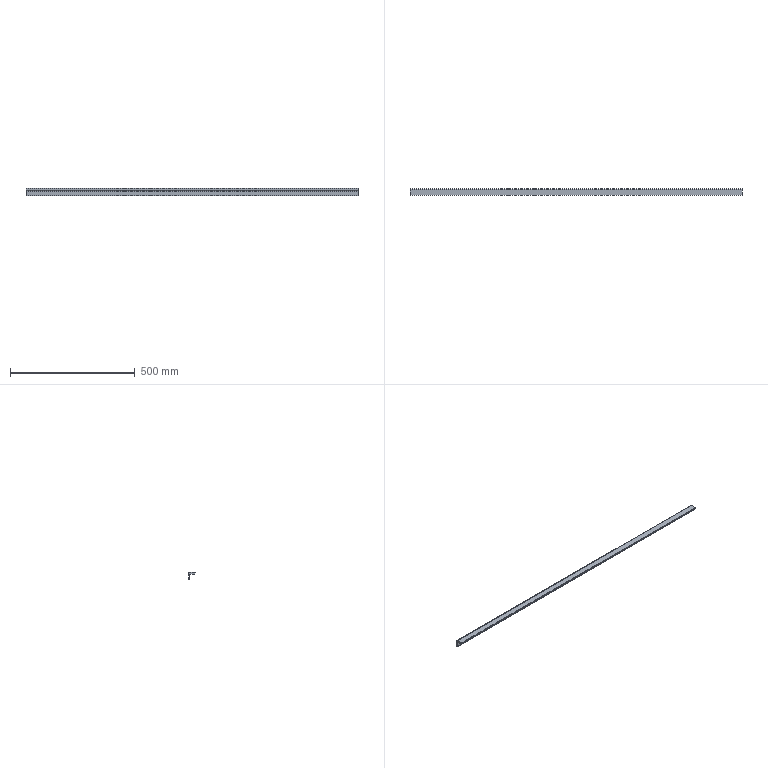Part | SolidWorks | features BaseBody 1 | 1 solid | 24 faces | box 1330 x 28 x 29.5 mm | volume 384644 mm3 | plane 19 | cylinder 5 | commonest cylinder face diameters 0.6 x3 8 x1 10 x1
STEP:
#1=CARTESIAN_POINT('',(-671.521,190.,396.5));
#2=VERTEX_POINT('',#1);
#3=CARTESIAN_POINT('',(-671.521,190.3,396.2));
#4=VERTEX_POINT('',#3);
#5=CARTESIAN_POINT('',(-671.521,190.3,396.5));
#6=DIRECTION('',(1.,0.,0.));
#7=DIRECTION('',(0.,0.,-1.));
#8=AXIS2_PLACEMENT_3D('',#5,#6,#7);
#9=CIRCLE('',#8,0.3);
#10=EDGE_CURVE('',#2,#4,#9,.T.);
#11=ORIENTED_EDGE('',*,*,#10,.T.);
#12=CARTESIAN_POINT('',(658.479,190.3,396.2));
#13=VERTEX_POINT('',#12);
#14=CARTESIAN_POINT('',(68.479,190.3,396.2));
#15=DIRECTION('',(1.,0.,0.));
#16=VECTOR('',#15,1000.);
#17=LINE('',#14,#16);
#18=EDGE_CURVE('',#4,#13,#17,.T.);
#19=ORIENTED_EDGE('',*,*,#18,.T.);
#20=CARTESIAN_POINT('',(658.479,190.,396.5));
#21=VERTEX_POINT('',#20);
#22=CARTESIAN_POINT('',(658.479,190.3,396.5));
#23=DIRECTION('',(1.,0.,0.));
#24=DIRECTION('',(0.,0.,-1.));
#25=AXIS2_PLACEMENT_3D('',#22,#23,#24);
#26=CIRCLE('',#25,0.3);
#27=EDGE_CURVE('',#21,#13,#26,.T.);
#28=ORIENTED_EDGE('',*,*,#27,.F.);
#29=CARTESIAN_POINT('',(68.479,190.,396.5));
#30=DIRECTION('',(-1.,0.,0.));
#31=VECTOR('',#30,1000.);
#32=LINE('',#29,#31);
#33=EDGE_CURVE('',#21,#2,#32,.T.);
#34=ORIENTED_EDGE('',*,*,#33,.T.);
#35=EDGE_LOOP('',(#11,#19,#28,#34));
#36=FACE_OUTER_BOUND('',#35,.T.);
#37=CARTESIAN_POINT('',(68.479,190.3,396.5));
#38=DIRECTION('',(1.,0.,0.));
#39=DIRECTION('',(0.,0.,-1.));
#40=AXIS2_PLACEMENT_3D('',#37,#38,#39);
#41=CYLINDRICAL_SURFACE('',#40,0.3);
#42=ADVANCED_FACE('',(#36),#41,.T.);
#43=CARTESIAN_POINT('',(658.479,187.,420.));
#44=VERTEX_POINT('',#43);
#45=CARTESIAN_POINT('',(-671.521,187.,420.));
#46=VERTEX_POINT('',#45);
#47=CARTESIAN_POINT('',(68.479,187.,420.));
#48=DIRECTION('',(-1.,0.,0.));
#49=VECTOR('',#48,1000.);
#50=LINE('',#47,#49);
#51=EDGE_CURVE('',#44,#46,#50,.T.);
#52=ORIENTED_EDGE('',*,*,#51,.T.);
#53=CARTESIAN_POINT('',(-671.521,164.,420.));
#54=VERTEX_POINT('',#53);
#55=CARTESIAN_POINT('',(-671.521,164.,420.));
#56=DIRECTION('',(0.,-1.,0.));
#57=VECTOR('',#56,1000.);
#58=LINE('',#55,#57);
#59=EDGE_CURVE('',#46,#54,#58,.T.);
#60=ORIENTED_EDGE('',*,*,#59,.T.);
#61=CARTESIAN_POINT('',(658.479,164.,420.));
#62=VERTEX_POINT('',#61);
#63=CARTESIAN_POINT('',(68.479,164.,420.));
#64=DIRECTION('',(1.,0.,0.));
#65=VECTOR('',#64,1000.);
#66=LINE('',#63,#65);
#67=EDGE_CURVE('',#54,#62,#66,.T.);
#68=ORIENTED_EDGE('',*,*,#67,.T.);
#69=CARTESIAN_POINT('',(658.479,164.,420.));
#70=DIRECTION('',(0.,1.,0.));
#71=VECTOR('',#70,1000.);
#72=LINE('',#69,#71);
#73=EDGE_CURVE('',#62,#44,#72,.T.);
#74=ORIENTED_EDGE('',*,*,#73,.T.);
#75=EDGE_LOOP('',(#52,#60,#68,#74));
#76=FACE_OUTER_BOUND('',#75,.T.);
#77=CARTESIAN_POINT('',(68.479,164.,420.));
#78=DIRECTION('',(0.,0.,1.));
#79=DIRECTION('',(0.,-1.,0.));
#80=AXIS2_PLACEMENT_3D('',#77,#78,#79);
#81=PLANE('',#80);
#82=ADVANCED_FACE('',(#76),#81,.T.);
#83=CARTESIAN_POINT('',(-671.521,164.,418.));
#84=VERTEX_POINT('',#83);
#85=CARTESIAN_POINT('',(-671.521,164.,408.659));
#86=DIRECTION('',(0.,0.,-1.));
#87=VECTOR('',#86,1000.);
#88=LINE('',#85,#87);
#89=EDGE_CURVE('',#54,#84,#88,.T.);
#90=ORIENTED_EDGE('',*,*,#89,.F.);
#91=ORIENTED_EDGE('',*,*,#59,.F.);
#92=CARTESIAN_POINT('',(-671.521,192.,415.));
#93=VERTEX_POINT('',#92);
#94=CARTESIAN_POINT('',(-671.521,187.,415.));
#95=DIRECTION('',(1.,0.,0.));
#96=DIRECTION('',(0.,0.,-1.));
#97=AXIS2_PLACEMENT_3D('',#94,#95,#96);
#98=CIRCLE('',#97,5.);
#99=EDGE_CURVE('',#93,#46,#98,.T.);
#100=ORIENTED_EDGE('',*,*,#99,.F.);
#101=CARTESIAN_POINT('',(-671.521,192.,400.7));
#102=VERTEX_POINT('',#101);
#103=CARTESIAN_POINT('',(-671.521,192.,408.659));
#104=DIRECTION('',(0.,0.,1.));
#105=VECTOR('',#104,1000.);
#106=LINE('',#103,#105);
#107=EDGE_CURVE('',#102,#93,#106,.T.);
#108=ORIENTED_EDGE('',*,*,#107,.F.);
#109=CARTESIAN_POINT('',(-671.521,191.8,400.5));
#110=VERTEX_POINT('',#109);
#111=CARTESIAN_POINT('',(-671.521,191.8,400.5));
#112=DIRECTION('',(0.,0.7071,0.7071));
#113=VECTOR('',#112,1000.);
#114=LINE('',#111,#113);
#115=EDGE_CURVE('',#110,#102,#114,.T.);
#116=ORIENTED_EDGE('',*,*,#115,.F.);
#117=CARTESIAN_POINT('',(-671.521,191.8,396.5));
#118=VERTEX_POINT('',#117);
#119=CARTESIAN_POINT('',(-671.521,191.8,408.659));
#120=DIRECTION('',(0.,0.,1.));
#121=VECTOR('',#120,1000.);
#122=LINE('',#119,#121);
#123=EDGE_CURVE('',#118,#110,#122,.T.);
#124=ORIENTED_EDGE('',*,*,#123,.F.);
#125=CARTESIAN_POINT('',(-671.521,190.6,396.5));
#126=VERTEX_POINT('',#125);
#127=CARTESIAN_POINT('',(-671.521,182.62,396.5));
#128=DIRECTION('',(0.,1.,0.));
#129=VECTOR('',#128,1000.);
#130=LINE('',#127,#129);
#131=EDGE_CURVE('',#126,#118,#130,.T.);
#132=ORIENTED_EDGE('',*,*,#131,.F.);
#133=CARTESIAN_POINT('',(-671.521,190.3,396.5));
#134=DIRECTION('',(1.,0.,0.));
#135=DIRECTION('',(0.,0.,-1.));
#136=AXIS2_PLACEMENT_3D('',#133,#134,#135);
#137=CIRCLE('',#136,0.3);
#138=EDGE_CURVE('',#4,#126,#137,.T.);
#139=ORIENTED_EDGE('',*,*,#138,.F.);
#140=ORIENTED_EDGE('',*,*,#10,.F.);
#141=CARTESIAN_POINT('',(-671.521,188.8,396.5));
#142=VERTEX_POINT('',#141);
#143=CARTESIAN_POINT('',(-671.521,182.62,396.5));
#144=DIRECTION('',(0.,1.,0.));
#145=VECTOR('',#144,1000.);
#146=LINE('',#143,#145);
#147=EDGE_CURVE('',#142,#2,#146,.T.);
#148=ORIENTED_EDGE('',*,*,#147,.F.);
#149=CARTESIAN_POINT('',(-671.521,188.8,392.5));
#150=VERTEX_POINT('',#149);
#151=CARTESIAN_POINT('',(-671.521,188.8,408.659));
#152=DIRECTION('',(0.,0.,1.));
#153=VECTOR('',#152,1000.);
#154=LINE('',#151,#153);
#155=EDGE_CURVE('',#150,#142,#154,.T.);
#156=ORIENTED_EDGE('',*,*,#155,.F.);
#157=CARTESIAN_POINT('',(-671.521,190.,392.5));
#158=VERTEX_POINT('',#157);
#159=CARTESIAN_POINT('',(-671.521,182.62,392.5));
#160=DIRECTION('',(0.,-1.,0.));
#161=VECTOR('',#160,1000.);
#162=LINE('',#159,#161);
#163=EDGE_CURVE('',#158,#150,#162,.T.);
#164=ORIENTED_EDGE('',*,*,#163,.F.);
#165=CARTESIAN_POINT('',(-671.521,190.6,392.5));
#166=VERTEX_POINT('',#165);
#167=CARTESIAN_POINT('',(-671.521,190.3,392.5));
#168=DIRECTION('',(1.,0.,0.));
#169=DIRECTION('',(0.,0.,-1.));
#170=AXIS2_PLACEMENT_3D('',#167,#168,#169);
#171=CIRCLE('',#170,0.3);
#172=EDGE_CURVE('',#166,#158,#171,.T.);
#173=ORIENTED_EDGE('',*,*,#172,.F.);
#174=CARTESIAN_POINT('',(-671.521,191.8,392.5));
#175=VERTEX_POINT('',#174);
#176=CARTESIAN_POINT('',(-671.521,182.62,392.5));
#177=DIRECTION('',(0.,-1.,0.));
#178=VECTOR('',#177,1000.);
#179=LINE('',#176,#178);
#180=EDGE_CURVE('',#175,#166,#179,.T.);
#181=ORIENTED_EDGE('',*,*,#180,.F.);
#182=CARTESIAN_POINT('',(-671.521,191.8,390.5));
#183=VERTEX_POINT('',#182);
#184=CARTESIAN_POINT('',(-671.521,191.8,408.659));
#185=DIRECTION('',(0.,0.,1.));
#186=VECTOR('',#185,1000.);
#187=LINE('',#184,#186);
#188=EDGE_CURVE('',#183,#175,#187,.T.);
#189=ORIENTED_EDGE('',*,*,#188,.F.);
#190=CARTESIAN_POINT('',(-671.521,187.,390.5));
#191=VERTEX_POINT('',#190);
#192=CARTESIAN_POINT('',(-671.521,182.62,390.5));
#193=DIRECTION('',(0.,1.,0.));
#194=VECTOR('',#193,1000.);
#195=LINE('',#192,#194);
#196=EDGE_CURVE('',#191,#183,#195,.T.);
#197=ORIENTED_EDGE('',*,*,#196,.F.);
#198=CARTESIAN_POINT('',(-671.521,187.,408.5));
#199=VERTEX_POINT('',#198);
#200=CARTESIAN_POINT('',(-671.521,187.,408.659));
#201=DIRECTION('',(0.,0.,-1.));
#202=VECTOR('',#201,1000.);
#203=LINE('',#200,#202);
#204=EDGE_CURVE('',#199,#191,#203,.T.);
#205=ORIENTED_EDGE('',*,*,#204,.F.);
#206=CARTESIAN_POINT('',(-671.521,183.,412.5));
#207=VERTEX_POINT('',#206);
#208=CARTESIAN_POINT('',(-671.521,183.,408.5));
#209=DIRECTION('',(-1.,0.,0.));
#210=DIRECTION('',(0.,0.,-1.));
#211=AXIS2_PLACEMENT_3D('',#208,#209,#210);
#212=CIRCLE('',#211,4.);
#213=EDGE_CURVE('',#207,#199,#212,.T.);
#214=ORIENTED_EDGE('',*,*,#213,.F.);
#215=CARTESIAN_POINT('',(-671.521,167.,412.5));
#216=VERTEX_POINT('',#215);
#217=CARTESIAN_POINT('',(-671.521,182.62,412.5));
#218=DIRECTION('',(0.,1.,0.));
#219=VECTOR('',#218,1000.);
#220=LINE('',#217,#219);
#221=EDGE_CURVE('',#216,#207,#220,.T.);
#222=ORIENTED_EDGE('',*,*,#221,.F.);
#223=CARTESIAN_POINT('',(-671.521,167.,417.5));
#224=VERTEX_POINT('',#223);
#225=CARTESIAN_POINT('',(-671.521,167.,408.659));
#226=DIRECTION('',(0.,0.,-1.));
#227=VECTOR('',#226,1000.);
#228=LINE('',#225,#227);
#229=EDGE_CURVE('',#224,#216,#228,.T.);
#230=ORIENTED_EDGE('',*,*,#229,.F.);
#231=CARTESIAN_POINT('',(-671.521,164.5,417.5));
#232=VERTEX_POINT('',#231);
#233=CARTESIAN_POINT('',(-671.521,182.62,417.5));
#234=DIRECTION('',(0.,1.,0.));
#235=VECTOR('',#234,1000.);
#236=LINE('',#233,#235);
#237=EDGE_CURVE('',#232,#224,#236,.T.);
#238=ORIENTED_EDGE('',*,*,#237,.F.);
#239=CARTESIAN_POINT('',(-671.521,164.,418.));
#240=DIRECTION('',(0.,0.7071,-0.7071));
#241=VECTOR('',#240,1000.);
#242=LINE('',#239,#241);
#243=EDGE_CURVE('',#84,#232,#242,.T.);
#244=ORIENTED_EDGE('',*,*,#243,.F.);
#245=EDGE_LOOP('',(#90,#91,#100,#108,#116,#124,#132,#139,#140,#148,#156,#164,#173,#181,#189,#197,#205,#214,#222,#230,#238,#244));
#246=FACE_OUTER_BOUND('',#245,.T.);
#247=CARTESIAN_POINT('',(-671.521,182.62,408.659));
#248=DIRECTION('',(1.,0.,0.));
#249=DIRECTION('',(0.,0.,-1.));
#250=AXIS2_PLACEMENT_3D('',#247,#248,#249);
#251=PLANE('',#250);
#252=ADVANCED_FACE('',(#246),#251,.F.);
#253=CARTESIAN_POINT('',(658.479,192.,415.));
#254=VERTEX_POINT('',#253);
#255=CARTESIAN_POINT('',(68.479,192.,415.));
#256=DIRECTION('',(-1.,0.,0.));
#257=VECTOR('',#256,1000.);
#258=LINE('',#255,#257);
#259=EDGE_CURVE('',#254,#93,#258,.T.);
#260=ORIENTED_EDGE('',*,*,#259,.T.);
#261=ORIENTED_EDGE('',*,*,#99,.T.);
#262=ORIENTED_EDGE('',*,*,#51,.F.);
#263=CARTESIAN_POINT('',(658.479,187.,415.));
#264=DIRECTION('',(-1.,0.,0.));
#265=DIRECTION('',(0.,0.,-1.));
#266=AXIS2_PLACEMENT_3D('',#263,#264,#265);
#267=CIRCLE('',#266,5.);
#268=EDGE_CURVE('',#44,#254,#267,.T.);
#269=ORIENTED_EDGE('',*,*,#268,.T.);
#270=EDGE_LOOP('',(#260,#261,#262,#269));
#271=FACE_OUTER_BOUND('',#270,.T.);
#272=CARTESIAN_POINT('',(68.479,187.,415.));
#273=DIRECTION('',(1.,0.,0.));
#274=DIRECTION('',(0.,0.,-1.));
#275=AXIS2_PLACEMENT_3D('',#272,#273,#274);
#276=CYLINDRICAL_SURFACE('',#275,5.);
#277=ADVANCED_FACE('',(#271),#276,.T.);
#278=ORIENTED_EDGE('',*,*,#73,.F.);
#279=CARTESIAN_POINT('',(658.479,164.,418.));
#280=VERTEX_POINT('',#279);
#281=CARTESIAN_POINT('',(658.479,164.,408.659));
#282=DIRECTION('',(0.,0.,-1.));
#283=VECTOR('',#282,1000.);
#284=LINE('',#281,#283);
#285=EDGE_CURVE('',#62,#280,#284,.T.);
#286=ORIENTED_EDGE('',*,*,#285,.T.);
#287=CARTESIAN_POINT('',(658.479,164.5,417.5));
#288=VERTEX_POINT('',#287);
#289=CARTESIAN_POINT('',(658.479,164.,418.));
#290=DIRECTION('',(0.,0.7071,-0.7071));
#291=VECTOR('',#290,1000.);
#292=LINE('',#289,#291);
#293=EDGE_CURVE('',#280,#288,#292,.T.);
#294=ORIENTED_EDGE('',*,*,#293,.T.);
#295=CARTESIAN_POINT('',(658.479,167.,417.5));
#296=VERTEX_POINT('',#295);
#297=CARTESIAN_POINT('',(658.479,182.62,417.5));
#298=DIRECTION('',(0.,1.,0.));
#299=VECTOR('',#298,1000.);
#300=LINE('',#297,#299);
#301=EDGE_CURVE('',#288,#296,#300,.T.);
#302=ORIENTED_EDGE('',*,*,#301,.T.);
#303=CARTESIAN_POINT('',(658.479,167.,412.5));
#304=VERTEX_POINT('',#303);
#305=CARTESIAN_POINT('',(658.479,167.,408.659));
#306=DIRECTION('',(0.,0.,-1.));
#307=VECTOR('',#306,1000.);
#308=LINE('',#305,#307);
#309=EDGE_CURVE('',#296,#304,#308,.T.);
#310=ORIENTED_EDGE('',*,*,#309,.T.);
#311=CARTESIAN_POINT('',(658.479,183.,412.5));
#312=VERTEX_POINT('',#311);
#313=CARTESIAN_POINT('',(658.479,182.62,412.5));
#314=DIRECTION('',(0.,1.,0.));
#315=VECTOR('',#314,1000.);
#316=LINE('',#313,#315);
#317=EDGE_CURVE('',#304,#312,#316,.T.);
#318=ORIENTED_EDGE('',*,*,#317,.T.);
#319=CARTESIAN_POINT('',(658.479,187.,408.5));
#320=VERTEX_POINT('',#319);
#321=CARTESIAN_POINT('',(658.479,183.,408.5));
#322=DIRECTION('',(-1.,0.,0.));
#323=DIRECTION('',(0.,0.,-1.));
#324=AXIS2_PLACEMENT_3D('',#321,#322,#323);
#325=CIRCLE('',#324,4.);
#326=EDGE_CURVE('',#312,#320,#325,.T.);
#327=ORIENTED_EDGE('',*,*,#326,.T.);
#328=CARTESIAN_POINT('',(658.479,187.,390.5));
#329=VERTEX_POINT('',#328);
#330=CARTESIAN_POINT('',(658.479,187.,408.659));
#331=DIRECTION('',(0.,0.,-1.));
#332=VECTOR('',#331,1000.);
#333=LINE('',#330,#332);
#334=EDGE_CURVE('',#320,#329,#333,.T.);
#335=ORIENTED_EDGE('',*,*,#334,.T.);
#336=CARTESIAN_POINT('',(658.479,191.8,390.5));
#337=VERTEX_POINT('',#336);
#338=CARTESIAN_POINT('',(658.479,182.62,390.5));
#339=DIRECTION('',(0.,1.,0.));
#340=VECTOR('',#339,1000.);
#341=LINE('',#338,#340);
#342=EDGE_CURVE('',#329,#337,#341,.T.);
#343=ORIENTED_EDGE('',*,*,#342,.T.);
#344=CARTESIAN_POINT('',(658.479,191.8,392.5));
#345=VERTEX_POINT('',#344);
#346=CARTESIAN_POINT('',(658.479,191.8,408.659));
#347=DIRECTION('',(0.,0.,1.));
#348=VECTOR('',#347,1000.);
#349=LINE('',#346,#348);
#350=EDGE_CURVE('',#337,#345,#349,.T.);
#351=ORIENTED_EDGE('',*,*,#350,.T.);
#352=CARTESIAN_POINT('',(658.479,190.6,392.5));
#353=VERTEX_POINT('',#352);
#354=CARTESIAN_POINT('',(658.479,182.62,392.5));
#355=DIRECTION('',(0.,-1.,0.));
#356=VECTOR('',#355,1000.);
#357=LINE('',#354,#356);
#358=EDGE_CURVE('',#345,#353,#357,.T.);
#359=ORIENTED_EDGE('',*,*,#358,.T.);
#360=CARTESIAN_POINT('',(658.479,190.,392.5));
#361=VERTEX_POINT('',#360);
#362=CARTESIAN_POINT('',(658.479,190.3,392.5));
#363=DIRECTION('',(1.,0.,0.));
#364=DIRECTION('',(0.,0.,-1.));
#365=AXIS2_PLACEMENT_3D('',#362,#363,#364);
#366=CIRCLE('',#365,0.3);
#367=EDGE_CURVE('',#353,#361,#366,.T.);
#368=ORIENTED_EDGE('',*,*,#367,.T.);
#369=CARTESIAN_POINT('',(658.479,188.8,392.5));
#370=VERTEX_POINT('',#369);
#371=CARTESIAN_POINT('',(658.479,182.62,392.5));
#372=DIRECTION('',(0.,-1.,0.));
#373=VECTOR('',#372,1000.);
#374=LINE('',#371,#373);
#375=EDGE_CURVE('',#361,#370,#374,.T.);
#376=ORIENTED_EDGE('',*,*,#375,.T.);
#377=CARTESIAN_POINT('',(658.479,188.8,396.5));
#378=VERTEX_POINT('',#377);
#379=CARTESIAN_POINT('',(658.479,188.8,408.659));
#380=DIRECTION('',(0.,0.,1.));
#381=VECTOR('',#380,1000.);
#382=LINE('',#379,#381);
#383=EDGE_CURVE('',#370,#378,#382,.T.);
#384=ORIENTED_EDGE('',*,*,#383,.T.);
#385=CARTESIAN_POINT('',(658.479,182.62,396.5));
#386=DIRECTION('',(0.,1.,0.));
#387=VECTOR('',#386,1000.);
#388=LINE('',#385,#387);
#389=EDGE_CURVE('',#378,#21,#388,.T.);
#390=ORIENTED_EDGE('',*,*,#389,.T.);
#391=ORIENTED_EDGE('',*,*,#27,.T.);
#392=CARTESIAN_POINT('',(658.479,190.6,396.5));
#393=VERTEX_POINT('',#392);
#394=CARTESIAN_POINT('',(658.479,190.3,396.5));
#395=DIRECTION('',(1.,0.,0.));
#396=DIRECTION('',(0.,0.,-1.));
#397=AXIS2_PLACEMENT_3D('',#394,#395,#396);
#398=CIRCLE('',#397,0.3);
#399=EDGE_CURVE('',#13,#393,#398,.T.);
#400=ORIENTED_EDGE('',*,*,#399,.T.);
#401=CARTESIAN_POINT('',(658.479,191.8,396.5));
#402=VERTEX_POINT('',#401);
#403=CARTESIAN_POINT('',(658.479,182.62,396.5));
#404=DIRECTION('',(0.,1.,0.));
#405=VECTOR('',#404,1000.);
#406=LINE('',#403,#405);
#407=EDGE_CURVE('',#393,#402,#406,.T.);
#408=ORIENTED_EDGE('',*,*,#407,.T.);
#409=CARTESIAN_POINT('',(658.479,191.8,400.5));
#410=VERTEX_POINT('',#409);
#411=CARTESIAN_POINT('',(658.479,191.8,408.659));
#412=DIRECTION('',(0.,0.,1.));
#413=VECTOR('',#412,1000.);
#414=LINE('',#411,#413);
#415=EDGE_CURVE('',#402,#410,#414,.T.);
#416=ORIENTED_EDGE('',*,*,#415,.T.);
#417=CARTESIAN_POINT('',(658.479,192.,400.7));
#418=VERTEX_POINT('',#417);
#419=CARTESIAN_POINT('',(658.479,191.8,400.5));
#420=DIRECTION('',(0.,0.7071,0.7071));
#421=VECTOR('',#420,1000.);
#422=LINE('',#419,#421);
#423=EDGE_CURVE('',#410,#418,#422,.T.);
#424=ORIENTED_EDGE('',*,*,#423,.T.);
#425=CARTESIAN_POINT('',(658.479,192.,408.659));
#426=DIRECTION('',(0.,0.,1.));
#427=VECTOR('',#426,1000.);
#428=LINE('',#425,#427);
#429=EDGE_CURVE('',#418,#254,#428,.T.);
#430=ORIENTED_EDGE('',*,*,#429,.T.);
#431=ORIENTED_EDGE('',*,*,#268,.F.);
#432=EDGE_LOOP('',(#278,#286,#294,#302,#310,#318,#327,#335,#343,#351,#359,#368,#376,#384,#390,#391,#400,#408,#416,#424,#430,#431));
#433=FACE_OUTER_BOUND('',#432,.T.);
#434=CARTESIAN_POINT('',(658.479,182.62,408.659));
#435=DIRECTION('',(1.,0.,0.));
#436=DIRECTION('',(0.,0.,-1.));
#437=AXIS2_PLACEMENT_3D('',#434,#435,#436);
#438=PLANE('',#437);
#439=ADVANCED_FACE('',(#433),#438,.T.);
#440=ORIENTED_EDGE('',*,*,#67,.F.);
#441=ORIENTED_EDGE('',*,*,#89,.T.);
#442=CARTESIAN_POINT('',(68.479,164.,418.));
#443=DIRECTION('',(1.,0.,0.));
#444=VECTOR('',#443,1000.);
#445=LINE('',#442,#444);
#446=EDGE_CURVE('',#84,#280,#445,.T.);
#447=ORIENTED_EDGE('',*,*,#446,.T.);
#448=ORIENTED_EDGE('',*,*,#285,.F.);
#449=EDGE_LOOP('',(#440,#441,#447,#448));
#450=FACE_OUTER_BOUND('',#449,.T.);
#451=CARTESIAN_POINT('',(68.479,164.,418.));
#452=DIRECTION('',(0.,-1.,0.));
#453=DIRECTION('',(0.,0.,-1.));
#454=AXIS2_PLACEMENT_3D('',#451,#452,#453);
#455=PLANE('',#454);
#456=ADVANCED_FACE('',(#450),#455,.T.);
#457=ORIENTED_EDGE('',*,*,#446,.F.);
#458=ORIENTED_EDGE('',*,*,#243,.T.);
#459=CARTESIAN_POINT('',(68.479,164.5,417.5));
#460=DIRECTION('',(1.,0.,0.));
#461=VECTOR('',#460,1000.);
#462=LINE('',#459,#461);
#463=EDGE_CURVE('',#232,#288,#462,.T.);
#464=ORIENTED_EDGE('',*,*,#463,.T.);
#465=ORIENTED_EDGE('',*,*,#293,.F.);
#466=EDGE_LOOP('',(#457,#458,#464,#465));
#467=FACE_OUTER_BOUND('',#466,.T.);
#468=CARTESIAN_POINT('',(68.479,164.5,417.5));
#469=DIRECTION('',(0.,-0.7071,-0.7071));
#470=DIRECTION('',(0.,0.7071,-0.7071));
#471=AXIS2_PLACEMENT_3D('',#468,#469,#470);
#472=PLANE('',#471);
#473=ADVANCED_FACE('',(#467),#472,.T.);
#474=CARTESIAN_POINT('',(68.479,192.,400.7));
#475=DIRECTION('',(-1.,0.,0.));
#476=VECTOR('',#475,1000.);
#477=LINE('',#474,#476);
#478=EDGE_CURVE('',#418,#102,#477,.T.);
#479=ORIENTED_EDGE('',*,*,#478,.T.);
#480=ORIENTED_EDGE('',*,*,#107,.T.);
#481=ORIENTED_EDGE('',*,*,#259,.F.);
#482=ORIENTED_EDGE('',*,*,#429,.F.);
#483=EDGE_LOOP('',(#479,#480,#481,#482));
#484=FACE_OUTER_BOUND('',#483,.T.);
#485=CARTESIAN_POINT('',(68.479,192.,415.));
#486=DIRECTION('',(0.,1.,0.));
#487=DIRECTION('',(0.,0.,1.));
#488=AXIS2_PLACEMENT_3D('',#485,#486,#487);
#489=PLANE('',#488);
#490=ADVANCED_FACE('',(#484),#489,.T.);
#491=CARTESIAN_POINT('',(68.479,191.8,400.5));
#492=DIRECTION('',(-1.,0.,0.));
#493=VECTOR('',#492,1000.);
#494=LINE('',#491,#493);
#495=EDGE_CURVE('',#410,#110,#494,.T.);
#496=ORIENTED_EDGE('',*,*,#495,.T.);
#497=ORIENTED_EDGE('',*,*,#115,.T.);
#498=ORIENTED_EDGE('',*,*,#478,.F.);
#499=ORIENTED_EDGE('',*,*,#423,.F.);
#500=EDGE_LOOP('',(#496,#497,#498,#499));
#501=FACE_OUTER_BOUND('',#500,.T.);
#502=CARTESIAN_POINT('',(68.479,192.,400.7));
#503=DIRECTION('',(0.,0.7071,-0.7071));
#504=DIRECTION('',(0.,0.7071,0.7071));
#505=AXIS2_PLACEMENT_3D('',#502,#503,#504);
#506=PLANE('',#505);
#507=ADVANCED_FACE('',(#501),#506,.T.);
#508=CARTESIAN_POINT('',(68.479,191.8,396.5));
#509=DIRECTION('',(-1.,0.,0.));
#510=VECTOR('',#509,1000.);
#511=LINE('',#508,#510);
#512=EDGE_CURVE('',#402,#118,#511,.T.);
#513=ORIENTED_EDGE('',*,*,#512,.T.);
#514=ORIENTED_EDGE('',*,*,#123,.T.);
#515=ORIENTED_EDGE('',*,*,#495,.F.);
#516=ORIENTED_EDGE('',*,*,#415,.F.);
#517=EDGE_LOOP('',(#513,#514,#515,#516));
#518=FACE_OUTER_BOUND('',#517,.T.);
#519=CARTESIAN_POINT('',(68.479,191.8,400.5));
#520=DIRECTION('',(0.,1.,0.));
#521=DIRECTION('',(0.,0.,1.));
#522=AXIS2_PLACEMENT_3D('',#519,#520,#521);
#523=PLANE('',#522);
#524=ADVANCED_FACE('',(#518),#523,.T.);
#525=CARTESIAN_POINT('',(68.479,190.6,396.5));
#526=DIRECTION('',(-1.,0.,0.));
#527=VECTOR('',#526,1000.);
#528=LINE('',#525,#527);
#529=EDGE_CURVE('',#393,#126,#528,.T.);
#530=ORIENTED_EDGE('',*,*,#529,.T.);
#531=ORIENTED_EDGE('',*,*,#131,.T.);
#532=ORIENTED_EDGE('',*,*,#512,.F.);
#533=ORIENTED_EDGE('',*,*,#407,.F.);
#534=EDGE_LOOP('',(#530,#531,#532,#533));
#535=FACE_OUTER_BOUND('',#534,.T.);
#536=CARTESIAN_POINT('',(68.479,191.8,396.5));
#537=DIRECTION('',(0.,0.,-1.));
#538=DIRECTION('',(-1.,0.,0.));
#539=AXIS2_PLACEMENT_3D('',#536,#537,#538);
#540=PLANE('',#539);
#541=ADVANCED_FACE('',(#535),#540,.T.);
#542=ORIENTED_EDGE('',*,*,#18,.F.);
#543=ORIENTED_EDGE('',*,*,#138,.T.);
#544=ORIENTED_EDGE('',*,*,#529,.F.);
#545=ORIENTED_EDGE('',*,*,#399,.F.);
#546=EDGE_LOOP('',(#542,#543,#544,#545));
#547=FACE_OUTER_BOUND('',#546,.T.);
#548=CARTESIAN_POINT('',(68.479,190.3,396.5));
#549=DIRECTION('',(1.,0.,0.));
#550=DIRECTION('',(0.,0.,-1.));
#551=AXIS2_PLACEMENT_3D('',#548,#549,#550);
#552=CYLINDRICAL_SURFACE('',#551,0.3);
#553=ADVANCED_FACE('',(#547),#552,.T.);
#554=CARTESIAN_POINT('',(68.479,188.8,396.5));
#555=DIRECTION('',(-1.,0.,0.));
#556=VECTOR('',#555,1000.);
#557=LINE('',#554,#556);
#558=EDGE_CURVE('',#378,#142,#557,.T.);
#559=ORIENTED_EDGE('',*,*,#558,.T.);
#560=ORIENTED_EDGE('',*,*,#147,.T.);
#561=ORIENTED_EDGE('',*,*,#33,.F.);
#562=ORIENTED_EDGE('',*,*,#389,.F.);
#563=EDGE_LOOP('',(#559,#560,#561,#562));
#564=FACE_OUTER_BOUND('',#563,.T.);
#565=CARTESIAN_POINT('',(68.479,190.,396.5));
#566=DIRECTION('',(0.,0.,-1.));
#567=DIRECTION('',(-1.,0.,0.));
#568=AXIS2_PLACEMENT_3D('',#565,#566,#567);
#569=PLANE('',#568);
#570=ADVANCED_FACE('',(#564),#569,.T.);
#571=CARTESIAN_POINT('',(68.479,188.8,392.5));
#572=DIRECTION('',(-1.,0.,0.));
#573=VECTOR('',#572,1000.);
#574=LINE('',#571,#573);
#575=EDGE_CURVE('',#370,#150,#574,.T.);
#576=ORIENTED_EDGE('',*,*,#575,.T.);
#577=ORIENTED_EDGE('',*,*,#155,.T.);
#578=ORIENTED_EDGE('',*,*,#558,.F.);
#579=ORIENTED_EDGE('',*,*,#383,.F.);
#580=EDGE_LOOP('',(#576,#577,#578,#579));
#581=FACE_OUTER_BOUND('',#580,.T.);
#582=CARTESIAN_POINT('',(68.479,188.8,396.5));
#583=DIRECTION('',(0.,1.,0.));
#584=DIRECTION('',(0.,0.,1.));
#585=AXIS2_PLACEMENT_3D('',#582,#583,#584);
#586=PLANE('',#585);
#587=ADVANCED_FACE('',(#581),#586,.T.);
#588=CARTESIAN_POINT('',(68.479,190.,392.5));
#589=DIRECTION('',(-1.,0.,0.));
#590=VECTOR('',#589,1000.);
#591=LINE('',#588,#590);
#592=EDGE_CURVE('',#361,#158,#591,.T.);
#593=ORIENTED_EDGE('',*,*,#592,.T.);
#594=ORIENTED_EDGE('',*,*,#163,.T.);
#595=ORIENTED_EDGE('',*,*,#575,.F.);
#596=ORIENTED_EDGE('',*,*,#375,.F.);
#597=EDGE_LOOP('',(#593,#594,#595,#596));
#598=FACE_OUTER_BOUND('',#597,.T.);
#599=CARTESIAN_POINT('',(68.479,188.8,392.5));
#600=DIRECTION('',(0.,0.,1.));
#601=DIRECTION('',(1.,0.,0.));
#602=AXIS2_PLACEMENT_3D('',#599,#600,#601);
#603=PLANE('',#602);
#604=ADVANCED_FACE('',(#598),#603,.T.);
#605=CARTESIAN_POINT('',(68.479,190.6,392.5));
#606=DIRECTION('',(-1.,0.,0.));
#607=VECTOR('',#606,1000.);
#608=LINE('',#605,#607);
#609=EDGE_CURVE('',#353,#166,#608,.T.);
#610=ORIENTED_EDGE('',*,*,#609,.T.);
#611=ORIENTED_EDGE('',*,*,#172,.T.);
#612=ORIENTED_EDGE('',*,*,#592,.F.);
#613=ORIENTED_EDGE('',*,*,#367,.F.);
#614=EDGE_LOOP('',(#610,#611,#612,#613));
#615=FACE_OUTER_BOUND('',#614,.T.);
#616=CARTESIAN_POINT('',(68.479,190.3,392.5));
#617=DIRECTION('',(1.,0.,0.));
#618=DIRECTION('',(0.,0.,-1.));
#619=AXIS2_PLACEMENT_3D('',#616,#617,#618);
#620=CYLINDRICAL_SURFACE('',#619,0.3);
#621=ADVANCED_FACE('',(#615),#620,.T.);
#622=CARTESIAN_POINT('',(68.479,191.8,392.5));
#623=DIRECTION('',(-1.,0.,0.));
#624=VECTOR('',#623,1000.);
#625=LINE('',#622,#624);
#626=EDGE_CURVE('',#345,#175,#625,.T.);
#627=ORIENTED_EDGE('',*,*,#626,.T.);
#628=ORIENTED_EDGE('',*,*,#180,.T.);
#629=ORIENTED_EDGE('',*,*,#609,.F.);
#630=ORIENTED_EDGE('',*,*,#358,.F.);
#631=EDGE_LOOP('',(#627,#628,#629,#630));
#632=FACE_OUTER_BOUND('',#631,.T.);
#633=CARTESIAN_POINT('',(68.479,190.6,392.5));
#634=DIRECTION('',(0.,0.,1.));
#635=DIRECTION('',(1.,0.,0.));
#636=AXIS2_PLACEMENT_3D('',#633,#634,#635);
#637=PLANE('',#636);
#638=ADVANCED_FACE('',(#632),#637,.T.);
#639=CARTESIAN_POINT('',(68.479,191.8,390.5));
#640=DIRECTION('',(-1.,0.,0.));
#641=VECTOR('',#640,1000.);
#642=LINE('',#639,#641);
#643=EDGE_CURVE('',#337,#183,#642,.T.);
#644=ORIENTED_EDGE('',*,*,#643,.T.);
#645=ORIENTED_EDGE('',*,*,#188,.T.);
#646=ORIENTED_EDGE('',*,*,#626,.F.);
#647=ORIENTED_EDGE('',*,*,#350,.F.);
#648=EDGE_LOOP('',(#644,#645,#646,#647));
#649=FACE_OUTER_BOUND('',#648,.T.);
#650=CARTESIAN_POINT('',(68.479,191.8,392.5));
#651=DIRECTION('',(0.,1.,0.));
#652=DIRECTION('',(0.,0.,1.));
#653=AXIS2_PLACEMENT_3D('',#650,#651,#652);
#654=PLANE('',#653);
#655=ADVANCED_FACE('',(#649),#654,.T.);
#656=CARTESIAN_POINT('',(68.479,187.,390.5));
#657=DIRECTION('',(-1.,0.,0.));
#658=VECTOR('',#657,1000.);
#659=LINE('',#656,#658);
#660=EDGE_CURVE('',#329,#191,#659,.T.);
#661=ORIENTED_EDGE('',*,*,#660,.T.);
#662=ORIENTED_EDGE('',*,*,#196,.T.);
#663=ORIENTED_EDGE('',*,*,#643,.F.);
#664=ORIENTED_EDGE('',*,*,#342,.F.);
#665=EDGE_LOOP('',(#661,#662,#663,#664));
#666=FACE_OUTER_BOUND('',#665,.T.);
#667=CARTESIAN_POINT('',(68.479,191.8,390.5));
#668=DIRECTION('',(0.,0.,-1.));
#669=DIRECTION('',(-1.,0.,0.));
#670=AXIS2_PLACEMENT_3D('',#667,#668,#669);
#671=PLANE('',#670);
#672=ADVANCED_FACE('',(#666),#671,.T.);
#673=CARTESIAN_POINT('',(68.479,187.,408.5));
#674=DIRECTION('',(-1.,0.,0.));
#675=VECTOR('',#674,1000.);
#676=LINE('',#673,#675);
#677=EDGE_CURVE('',#320,#199,#676,.T.);
#678=ORIENTED_EDGE('',*,*,#677,.T.);
#679=ORIENTED_EDGE('',*,*,#204,.T.);
#680=ORIENTED_EDGE('',*,*,#660,.F.);
#681=ORIENTED_EDGE('',*,*,#334,.F.);
#682=EDGE_LOOP('',(#678,#679,#680,#681));
#683=FACE_OUTER_BOUND('',#682,.T.);
#684=CARTESIAN_POINT('',(68.479,187.,390.5));
#685=DIRECTION('',(0.,-1.,0.));
#686=DIRECTION('',(0.,0.,-1.));
#687=AXIS2_PLACEMENT_3D('',#684,#685,#686);
#688=PLANE('',#687);
#689=ADVANCED_FACE('',(#683),#688,.T.);
#690=ORIENTED_EDGE('',*,*,#677,.F.);
#691=ORIENTED_EDGE('',*,*,#326,.F.);
#692=CARTESIAN_POINT('',(68.479,183.,412.5));
#693=DIRECTION('',(1.,0.,0.));
#694=VECTOR('',#693,1000.);
#695=LINE('',#692,#694);
#696=EDGE_CURVE('',#207,#312,#695,.T.);
#697=ORIENTED_EDGE('',*,*,#696,.F.);
#698=ORIENTED_EDGE('',*,*,#213,.T.);
#699=EDGE_LOOP('',(#690,#691,#697,#698));
#700=FACE_OUTER_BOUND('',#699,.T.);
#701=CARTESIAN_POINT('',(68.479,183.,408.5));
#702=DIRECTION('',(1.,0.,0.));
#703=DIRECTION('',(0.,0.,-1.));
#704=AXIS2_PLACEMENT_3D('',#701,#702,#703);
#705=CYLINDRICAL_SURFACE('',#704,4.);
#706=ADVANCED_FACE('',(#700),#705,.F.);
#707=CARTESIAN_POINT('',(68.479,167.,412.5));
#708=DIRECTION('',(-1.,0.,0.));
#709=VECTOR('',#708,1000.);
#710=LINE('',#707,#709);
#711=EDGE_CURVE('',#304,#216,#710,.T.);
#712=ORIENTED_EDGE('',*,*,#711,.T.);
#713=ORIENTED_EDGE('',*,*,#221,.T.);
#714=ORIENTED_EDGE('',*,*,#696,.T.);
#715=ORIENTED_EDGE('',*,*,#317,.F.);
#716=EDGE_LOOP('',(#712,#713,#714,#715));
#717=FACE_OUTER_BOUND('',#716,.T.);
#718=CARTESIAN_POINT('',(68.479,183.,412.5));
#719=DIRECTION('',(0.,0.,-1.));
#720=DIRECTION('',(0.,1.,0.));
#721=AXIS2_PLACEMENT_3D('',#718,#719,#720);
#722=PLANE('',#721);
#723=ADVANCED_FACE('',(#717),#722,.T.);
#724=CARTESIAN_POINT('',(68.479,167.,417.5));
#725=DIRECTION('',(-1.,0.,0.));
#726=VECTOR('',#725,1000.);
#727=LINE('',#724,#726);
#728=EDGE_CURVE('',#296,#224,#727,.T.);
#729=ORIENTED_EDGE('',*,*,#728,.T.);
#730=ORIENTED_EDGE('',*,*,#229,.T.);
#731=ORIENTED_EDGE('',*,*,#711,.F.);
#732=ORIENTED_EDGE('',*,*,#309,.F.);
#733=EDGE_LOOP('',(#729,#730,#731,#732));
#734=FACE_OUTER_BOUND('',#733,.T.);
#735=CARTESIAN_POINT('',(68.479,167.,412.5));
#736=DIRECTION('',(0.,-1.,0.));
#737=DIRECTION('',(0.,0.,-1.));
#738=AXIS2_PLACEMENT_3D('',#735,#736,#737);
#739=PLANE('',#738);
#740=ADVANCED_FACE('',(#734),#739,.T.);
#741=ORIENTED_EDGE('',*,*,#463,.F.);
#742=ORIENTED_EDGE('',*,*,#237,.T.);
#743=ORIENTED_EDGE('',*,*,#728,.F.);
#744=ORIENTED_EDGE('',*,*,#301,.F.);
#745=EDGE_LOOP('',(#741,#742,#743,#744));
#746=FACE_OUTER_BOUND('',#745,.T.);
#747=CARTESIAN_POINT('',(68.479,167.,417.5));
#748=DIRECTION('',(0.,0.,-1.));
#749=DIRECTION('',(0.,1.,0.));
#750=AXIS2_PLACEMENT_3D('',#747,#748,#749);
#751=PLANE('',#750);
#752=ADVANCED_FACE('',(#746),#751,.T.);
#753=CLOSED_SHELL('',(#42,#82,#252,#277,#439,#456,#473,#490,#507,#524,#541,#553,#570,#587,#604,#621,#638,#655,#672,#689,#706,#723,#740,#752));
#754=MANIFOLD_SOLID_BREP('',#753);
#755=CARTESIAN_POINT('',(0.,0.,0.));
#756=DIRECTION('',(0.,0.,1.));
#757=DIRECTION('',(1.,0.,0.));
#758=AXIS2_PLACEMENT_3D('',#755,#756,#757);
#759=(LENGTH_UNIT()NAMED_UNIT(*)SI_UNIT(.MILLI.,.METRE.));
#760=UNCERTAINTY_MEASURE_WITH_UNIT(LENGTH_MEASURE(0.00001),#759,'','');
#761=(NAMED_UNIT(*)PLANE_ANGLE_UNIT()SI_UNIT($,.RADIAN.));
#762=(NAMED_UNIT(*)SI_UNIT($,.STERADIAN.)SOLID_ANGLE_UNIT());
#763=(GEOMETRIC_REPRESENTATION_CONTEXT(3)GLOBAL_UNCERTAINTY_ASSIGNED_CONTEXT((#760))GLOBAL_UNIT_ASSIGNED_CONTEXT((#759,#761,#762))REPRESENTATION_CONTEXT('',''));
#764=ADVANCED_BREP_SHAPE_REPRESENTATION('',(#754,#758),#763);